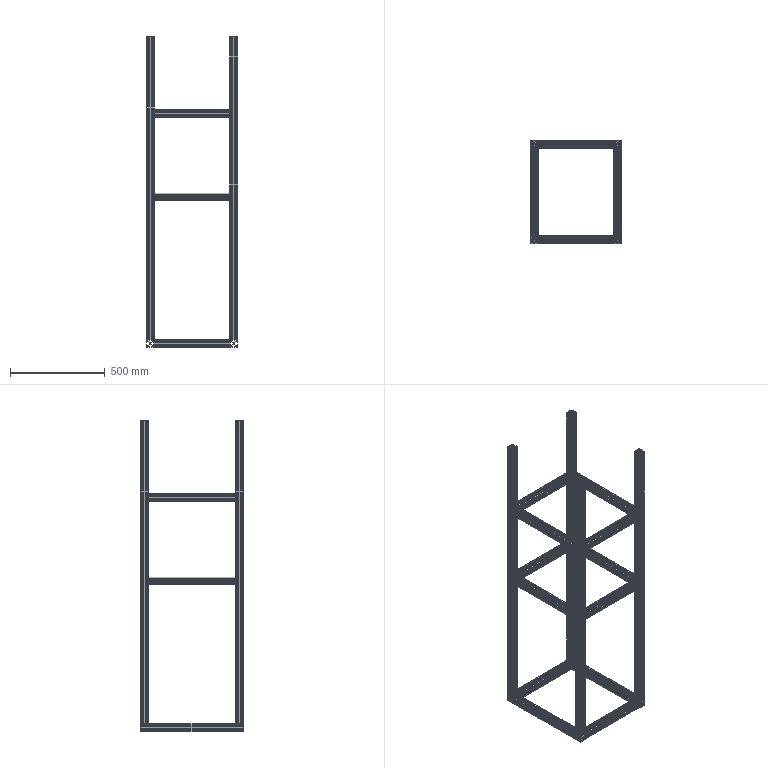Part | SolidWorks | features WeldCornerFeat 16, WeldMemberFeat 8, 3DProfileFeature 1, ICE 1, WeldmentFeature 1 | 20 solids | 2080 faces | box 480 x 540 x 1635 mm | volume 5554976 mm3 | plane 1880 | cylinder 200 | commonest cylinder face diameters 5 x80 9 x80 6.8 x40